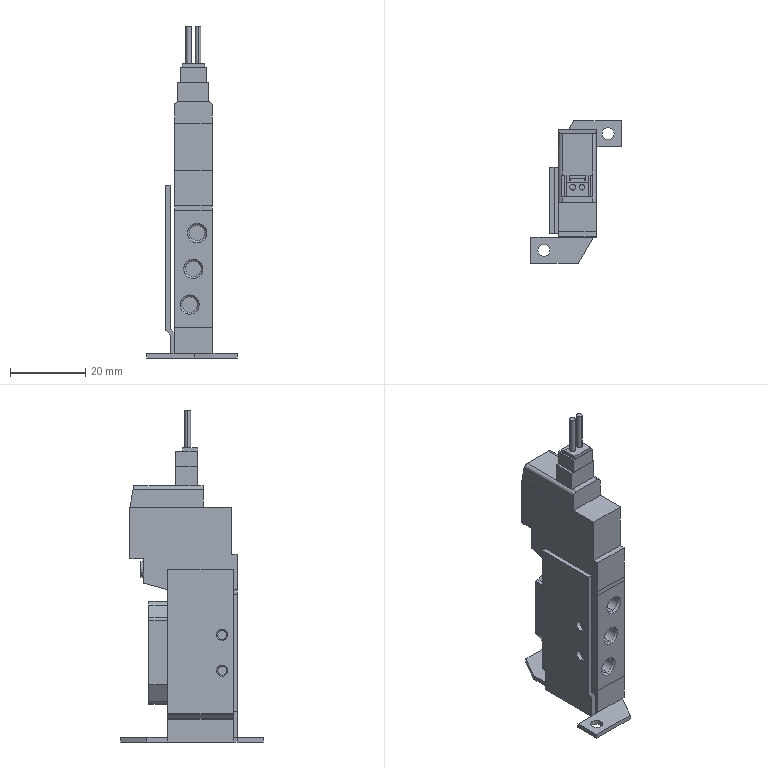Part | SolidWorks | features BaseBody 1 | 1 solid | 172 faces | box 24.041 x 38 x 88.25 mm | volume 16472 mm3 | plane 117 | cylinder 39 | cone 14 | spline 2 | commonest cylinder face diameters 4.13 x10 3.2 x7 1 x4 1.5 x4 2.46 x4 3 x4